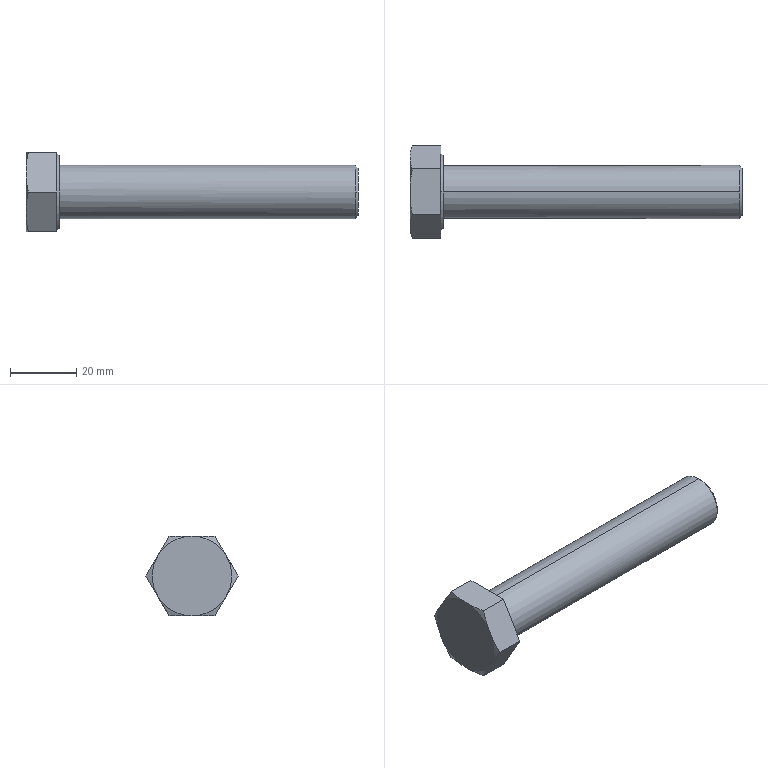Part | STEP file | hex head bolts-full thread grade c gb_GB_FASTENER_BOLT_HHBFTC M16X90-S | 1 solid | 22 faces | box 100 x 27.713 x 24 mm | volume 22987 mm3 | cone 10 | plane 10 | cylinder 2 | commonest cylinder face diameters 16 x2
STEP:
#1=CARTESIAN_POINT('',(99.2,8.,0.));
#2=VERTEX_POINT('',#1);
#3=CARTESIAN_POINT('',(99.2,0.,-8.));
#4=VERTEX_POINT('',#3);
#5=CARTESIAN_POINT('',(99.2,0.,0.));
#6=DIRECTION('',(-1.,0.,0.));
#7=DIRECTION('',(0.,0.,1.));
#8=AXIS2_PLACEMENT_3D('',#5,#6,#7);
#9=CIRCLE('',#8,8.);
#10=EDGE_CURVE('',#2,#4,#9,.T.);
#11=ORIENTED_EDGE('',*,*,#10,.T.);
#12=CARTESIAN_POINT('',(10.,0.,-8.));
#13=VERTEX_POINT('',#12);
#14=CARTESIAN_POINT('',(100.,0.,-8.));
#15=DIRECTION('',(-1.,0.,0.));
#16=VECTOR('',#15,1000.);
#17=LINE('',#14,#16);
#18=EDGE_CURVE('',#4,#13,#17,.T.);
#19=ORIENTED_EDGE('',*,*,#18,.T.);
#20=CARTESIAN_POINT('',(10.,0.,8.));
#21=VERTEX_POINT('',#20);
#22=CARTESIAN_POINT('',(10.,0.,0.));
#23=DIRECTION('',(1.,0.,0.));
#24=DIRECTION('',(0.,0.,1.));
#25=AXIS2_PLACEMENT_3D('',#22,#23,#24);
#26=CIRCLE('',#25,8.);
#27=EDGE_CURVE('',#13,#21,#26,.T.);
#28=ORIENTED_EDGE('',*,*,#27,.T.);
#29=CARTESIAN_POINT('',(99.2,0.,8.));
#30=VERTEX_POINT('',#29);
#31=CARTESIAN_POINT('',(100.,0.,8.));
#32=DIRECTION('',(-1.,0.,0.));
#33=VECTOR('',#32,1000.);
#34=LINE('',#31,#33);
#35=EDGE_CURVE('',#30,#21,#34,.T.);
#36=ORIENTED_EDGE('',*,*,#35,.F.);
#37=CARTESIAN_POINT('',(99.2,0.,0.));
#38=DIRECTION('',(-1.,0.,0.));
#39=DIRECTION('',(0.,0.,1.));
#40=AXIS2_PLACEMENT_3D('',#37,#38,#39);
#41=CIRCLE('',#40,8.);
#42=EDGE_CURVE('',#30,#2,#41,.T.);
#43=ORIENTED_EDGE('',*,*,#42,.T.);
#44=EDGE_LOOP('',(#11,#19,#28,#36,#43));
#45=FACE_OUTER_BOUND('',#44,.T.);
#46=CARTESIAN_POINT('',(100.,0.,0.));
#47=DIRECTION('',(-1.,0.,0.));
#48=DIRECTION('',(0.,0.,1.));
#49=AXIS2_PLACEMENT_3D('',#46,#47,#48);
#50=CYLINDRICAL_SURFACE('',#49,8.);
#51=ADVANCED_FACE('',(#45),#50,.T.);
#52=CARTESIAN_POINT('',(100.,-7.2,0.));
#53=VERTEX_POINT('',#52);
#54=CARTESIAN_POINT('',(100.,7.2,0.));
#55=VERTEX_POINT('',#54);
#56=CARTESIAN_POINT('',(100.,0.,0.));
#57=DIRECTION('',(-1.,0.,0.));
#58=DIRECTION('',(0.,-1.,0.));
#59=AXIS2_PLACEMENT_3D('',#56,#57,#58);
#60=CIRCLE('',#59,7.2);
#61=EDGE_CURVE('',#53,#55,#60,.T.);
#62=ORIENTED_EDGE('',*,*,#61,.T.);
#63=CARTESIAN_POINT('',(99.2,8.,0.));
#64=DIRECTION('',(-0.7071,0.7071,0.));
#65=VECTOR('',#64,1000.);
#66=LINE('',#63,#65);
#67=EDGE_CURVE('',#55,#2,#66,.T.);
#68=ORIENTED_EDGE('',*,*,#67,.T.);
#69=ORIENTED_EDGE('',*,*,#42,.F.);
#70=CARTESIAN_POINT('',(99.2,-8.,0.));
#71=VERTEX_POINT('',#70);
#72=CARTESIAN_POINT('',(99.2,0.,0.));
#73=DIRECTION('',(-1.,0.,0.));
#74=DIRECTION('',(0.,0.,1.));
#75=AXIS2_PLACEMENT_3D('',#72,#73,#74);
#76=CIRCLE('',#75,8.);
#77=EDGE_CURVE('',#71,#30,#76,.T.);
#78=ORIENTED_EDGE('',*,*,#77,.F.);
#79=CARTESIAN_POINT('',(99.2,-8.,0.));
#80=DIRECTION('',(-0.7071,-0.7071,0.));
#81=VECTOR('',#80,1000.);
#82=LINE('',#79,#81);
#83=EDGE_CURVE('',#53,#71,#82,.T.);
#84=ORIENTED_EDGE('',*,*,#83,.F.);
#85=EDGE_LOOP('',(#62,#68,#69,#78,#84));
#86=FACE_OUTER_BOUND('',#85,.T.);
#87=CARTESIAN_POINT('',(99.2,0.,0.));
#88=DIRECTION('',(-1.,0.,0.));
#89=DIRECTION('',(0.,-1.,0.));
#90=AXIS2_PLACEMENT_3D('',#87,#88,#89);
#91=CONICAL_SURFACE('',#90,8.,0.7854);
#92=ADVANCED_FACE('',(#86),#91,.T.);
#93=CARTESIAN_POINT('',(10.,0.,11.));
#94=VERTEX_POINT('',#93);
#95=CARTESIAN_POINT('',(10.,0.,-11.));
#96=VERTEX_POINT('',#95);
#97=CARTESIAN_POINT('',(10.,0.,0.));
#98=DIRECTION('',(-1.,0.,0.));
#99=DIRECTION('',(0.,0.,1.));
#100=AXIS2_PLACEMENT_3D('',#97,#98,#99);
#101=CIRCLE('',#100,11.);
#102=EDGE_CURVE('',#94,#96,#101,.T.);
#103=ORIENTED_EDGE('',*,*,#102,.T.);
#104=CARTESIAN_POINT('',(9.2,0.,-11.8));
#105=VERTEX_POINT('',#104);
#106=CARTESIAN_POINT('',(9.2,0.,-11.8));
#107=DIRECTION('',(-0.7071,0.,-0.7071));
#108=VECTOR('',#107,1000.);
#109=LINE('',#106,#108);
#110=EDGE_CURVE('',#96,#105,#109,.T.);
#111=ORIENTED_EDGE('',*,*,#110,.T.);
#112=CARTESIAN_POINT('',(9.2,0.,11.8));
#113=VERTEX_POINT('',#112);
#114=CARTESIAN_POINT('',(9.2,0.,0.));
#115=DIRECTION('',(1.,0.,0.));
#116=DIRECTION('',(0.,0.,1.));
#117=AXIS2_PLACEMENT_3D('',#114,#115,#116);
#118=CIRCLE('',#117,11.8);
#119=EDGE_CURVE('',#105,#113,#118,.T.);
#120=ORIENTED_EDGE('',*,*,#119,.T.);
#121=CARTESIAN_POINT('',(9.2,0.,11.8));
#122=DIRECTION('',(-0.7071,0.,0.7071));
#123=VECTOR('',#122,1000.);
#124=LINE('',#121,#123);
#125=EDGE_CURVE('',#94,#113,#124,.T.);
#126=ORIENTED_EDGE('',*,*,#125,.F.);
#127=EDGE_LOOP('',(#103,#111,#120,#126));
#128=FACE_OUTER_BOUND('',#127,.T.);
#129=CARTESIAN_POINT('',(9.2,0.,0.));
#130=DIRECTION('',(-1.,0.,0.));
#131=DIRECTION('',(0.,0.,1.));
#132=AXIS2_PLACEMENT_3D('',#129,#130,#131);
#133=CONICAL_SURFACE('',#132,11.8,0.7854);
#134=ADVANCED_FACE('',(#128),#133,.T.);
#135=ORIENTED_EDGE('',*,*,#18,.F.);
#136=CARTESIAN_POINT('',(99.2,0.,0.));
#137=DIRECTION('',(-1.,0.,0.));
#138=DIRECTION('',(0.,0.,1.));
#139=AXIS2_PLACEMENT_3D('',#136,#137,#138);
#140=CIRCLE('',#139,8.);
#141=EDGE_CURVE('',#4,#71,#140,.T.);
#142=ORIENTED_EDGE('',*,*,#141,.T.);
#143=ORIENTED_EDGE('',*,*,#77,.T.);
#144=ORIENTED_EDGE('',*,*,#35,.T.);
#145=CARTESIAN_POINT('',(10.,0.,0.));
#146=DIRECTION('',(1.,0.,0.));
#147=DIRECTION('',(0.,0.,1.));
#148=AXIS2_PLACEMENT_3D('',#145,#146,#147);
#149=CIRCLE('',#148,8.);
#150=EDGE_CURVE('',#21,#13,#149,.T.);
#151=ORIENTED_EDGE('',*,*,#150,.T.);
#152=EDGE_LOOP('',(#135,#142,#143,#144,#151));
#153=FACE_OUTER_BOUND('',#152,.T.);
#154=CARTESIAN_POINT('',(100.,0.,0.));
#155=DIRECTION('',(-1.,0.,0.));
#156=DIRECTION('',(0.,0.,1.));
#157=AXIS2_PLACEMENT_3D('',#154,#155,#156);
#158=CYLINDRICAL_SURFACE('',#157,8.);
#159=ADVANCED_FACE('',(#153),#158,.T.);
#160=ORIENTED_EDGE('',*,*,#150,.F.);
#161=ORIENTED_EDGE('',*,*,#27,.F.);
#162=EDGE_LOOP('',(#160,#161));
#163=FACE_BOUND('',#162,.T.);
#164=ORIENTED_EDGE('',*,*,#102,.F.);
#165=CARTESIAN_POINT('',(10.,0.,0.));
#166=DIRECTION('',(-1.,0.,0.));
#167=DIRECTION('',(0.,0.,1.));
#168=AXIS2_PLACEMENT_3D('',#165,#166,#167);
#169=CIRCLE('',#168,11.);
#170=EDGE_CURVE('',#96,#94,#169,.T.);
#171=ORIENTED_EDGE('',*,*,#170,.F.);
#172=EDGE_LOOP('',(#164,#171));
#173=FACE_OUTER_BOUND('',#172,.T.);
#174=CARTESIAN_POINT('',(10.,0.,24.));
#175=DIRECTION('',(-1.,0.,0.));
#176=DIRECTION('',(0.,0.,1.));
#177=AXIS2_PLACEMENT_3D('',#174,#175,#176);
#178=PLANE('',#177);
#179=ADVANCED_FACE('',(#163,#173),#178,.F.);
#180=ORIENTED_EDGE('',*,*,#67,.F.);
#181=CARTESIAN_POINT('',(100.,0.,0.));
#182=DIRECTION('',(-1.,0.,0.));
#183=DIRECTION('',(0.,-1.,0.));
#184=AXIS2_PLACEMENT_3D('',#181,#182,#183);
#185=CIRCLE('',#184,7.2);
#186=EDGE_CURVE('',#55,#53,#185,.T.);
#187=ORIENTED_EDGE('',*,*,#186,.T.);
#188=ORIENTED_EDGE('',*,*,#83,.T.);
#189=ORIENTED_EDGE('',*,*,#141,.F.);
#190=ORIENTED_EDGE('',*,*,#10,.F.);
#191=EDGE_LOOP('',(#180,#187,#188,#189,#190));
#192=FACE_OUTER_BOUND('',#191,.T.);
#193=CARTESIAN_POINT('',(99.2,0.,0.));
#194=DIRECTION('',(-1.,0.,0.));
#195=DIRECTION('',(0.,-1.,0.));
#196=AXIS2_PLACEMENT_3D('',#193,#194,#195);
#197=CONICAL_SURFACE('',#196,8.,0.7854);
#198=ADVANCED_FACE('',(#192),#197,.T.);
#199=ORIENTED_EDGE('',*,*,#110,.F.);
#200=ORIENTED_EDGE('',*,*,#170,.T.);
#201=ORIENTED_EDGE('',*,*,#125,.T.);
#202=CARTESIAN_POINT('',(9.2,0.,0.));
#203=DIRECTION('',(1.,0.,0.));
#204=DIRECTION('',(0.,0.,1.));
#205=AXIS2_PLACEMENT_3D('',#202,#203,#204);
#206=CIRCLE('',#205,11.8);
#207=EDGE_CURVE('',#113,#105,#206,.T.);
#208=ORIENTED_EDGE('',*,*,#207,.T.);
#209=EDGE_LOOP('',(#199,#200,#201,#208));
#210=FACE_OUTER_BOUND('',#209,.T.);
#211=CARTESIAN_POINT('',(9.2,0.,0.));
#212=DIRECTION('',(-1.,0.,0.));
#213=DIRECTION('',(0.,0.,1.));
#214=AXIS2_PLACEMENT_3D('',#211,#212,#213);
#215=CONICAL_SURFACE('',#214,11.8,0.7854);
#216=ADVANCED_FACE('',(#210),#215,.T.);
#217=ORIENTED_EDGE('',*,*,#61,.F.);
#218=ORIENTED_EDGE('',*,*,#186,.F.);
#219=EDGE_LOOP('',(#217,#218));
#220=FACE_OUTER_BOUND('',#219,.T.);
#221=CARTESIAN_POINT('',(100.,0.,0.));
#222=DIRECTION('',(1.,0.,0.));
#223=DIRECTION('',(0.,0.,-1.));
#224=AXIS2_PLACEMENT_3D('',#221,#222,#223);
#225=PLANE('',#224);
#226=ADVANCED_FACE('',(#220),#225,.T.);
#227=CARTESIAN_POINT('',(9.2,13.856,0.));
#228=VERTEX_POINT('',#227);
#229=CARTESIAN_POINT('',(9.2,6.928,12.));
#230=VERTEX_POINT('',#229);
#231=CARTESIAN_POINT('',(9.2,13.856,0.));
#232=DIRECTION('',(0.,-0.5,0.866));
#233=VECTOR('',#232,1000.);
#234=LINE('',#231,#233);
#235=EDGE_CURVE('',#228,#230,#234,.T.);
#236=ORIENTED_EDGE('',*,*,#235,.T.);
#237=CARTESIAN_POINT('',(9.2,-6.928,12.));
#238=VERTEX_POINT('',#237);
#239=CARTESIAN_POINT('',(9.2,11.8,12.));
#240=DIRECTION('',(0.,-1.,0.));
#241=VECTOR('',#240,1000.);
#242=LINE('',#239,#241);
#243=EDGE_CURVE('',#230,#238,#242,.T.);
#244=ORIENTED_EDGE('',*,*,#243,.T.);
#245=CARTESIAN_POINT('',(9.2,-13.856,0.));
#246=VERTEX_POINT('',#245);
#247=CARTESIAN_POINT('',(9.2,-6.928,12.));
#248=DIRECTION('',(0.,-0.5,-0.866));
#249=VECTOR('',#248,1000.);
#250=LINE('',#247,#249);
#251=EDGE_CURVE('',#238,#246,#250,.T.);
#252=ORIENTED_EDGE('',*,*,#251,.T.);
#253=CARTESIAN_POINT('',(9.2,-6.928,-12.));
#254=VERTEX_POINT('',#253);
#255=CARTESIAN_POINT('',(9.2,-13.856,0.));
#256=DIRECTION('',(0.,0.5,-0.866));
#257=VECTOR('',#256,1000.);
#258=LINE('',#255,#257);
#259=EDGE_CURVE('',#246,#254,#258,.T.);
#260=ORIENTED_EDGE('',*,*,#259,.T.);
#261=CARTESIAN_POINT('',(9.2,6.928,-12.));
#262=VERTEX_POINT('',#261);
#263=CARTESIAN_POINT('',(9.2,11.8,-12.));
#264=DIRECTION('',(0.,1.,0.));
#265=VECTOR('',#264,1000.);
#266=LINE('',#263,#265);
#267=EDGE_CURVE('',#254,#262,#266,.T.);
#268=ORIENTED_EDGE('',*,*,#267,.T.);
#269=CARTESIAN_POINT('',(9.2,6.928,-12.));
#270=DIRECTION('',(0.,0.5,0.866));
#271=VECTOR('',#270,1000.);
#272=LINE('',#269,#271);
#273=EDGE_CURVE('',#262,#228,#272,.T.);
#274=ORIENTED_EDGE('',*,*,#273,.T.);
#275=EDGE_LOOP('',(#236,#244,#252,#260,#268,#274));
#276=FACE_OUTER_BOUND('',#275,.T.);
#277=ORIENTED_EDGE('',*,*,#207,.F.);
#278=ORIENTED_EDGE('',*,*,#119,.F.);
#279=EDGE_LOOP('',(#277,#278));
#280=FACE_BOUND('',#279,.T.);
#281=CARTESIAN_POINT('',(9.2,11.8,0.));
#282=DIRECTION('',(1.,0.,0.));
#283=DIRECTION('',(0.,0.,-1.));
#284=AXIS2_PLACEMENT_3D('',#281,#282,#283);
#285=PLANE('',#284);
#286=ADVANCED_FACE('',(#276,#280),#285,.T.);
#287=CARTESIAN_POINT('',(0.6757,-6.928,12.));
#288=VERTEX_POINT('',#287);
#289=CARTESIAN_POINT('',(10.,-6.928,12.));
#290=DIRECTION('',(-1.,0.,0.));
#291=VECTOR('',#290,1000.);
#292=LINE('',#289,#291);
#293=EDGE_CURVE('',#238,#288,#292,.T.);
#294=ORIENTED_EDGE('',*,*,#293,.F.);
#295=ORIENTED_EDGE('',*,*,#243,.F.);
#296=CARTESIAN_POINT('',(0.6757,6.928,12.));
#297=VERTEX_POINT('',#296);
#298=CARTESIAN_POINT('',(10.,6.928,12.));
#299=DIRECTION('',(1.,0.,0.));
#300=VECTOR('',#299,1000.);
#301=LINE('',#298,#300);
#302=EDGE_CURVE('',#297,#230,#301,.T.);
#303=ORIENTED_EDGE('',*,*,#302,.F.);
#304=CARTESIAN_POINT('',(0.,0.,12.));
#305=VERTEX_POINT('',#304);
#306=CARTESIAN_POINT('',(0.,0.,12.));
#307=CARTESIAN_POINT('',(0.,1.166,12.));
#308=CARTESIAN_POINT('',(0.0629,2.325,12.));
#309=CARTESIAN_POINT('',(0.2969,4.634,12.));
#310=CARTESIAN_POINT('',(0.4672,5.783,12.));
#311=CARTESIAN_POINT('',(0.6757,6.928,12.));
#312=B_SPLINE_CURVE_WITH_KNOTS('',3,(#306,#307,#308,#309,#310,#311),.UNSPECIFIED.,.F.,.F.,(4,2,4),(0.,0.003481,0.006961),.UNSPECIFIED.);
#313=EDGE_CURVE('',#305,#297,#312,.T.);
#314=ORIENTED_EDGE('',*,*,#313,.F.);
#315=CARTESIAN_POINT('',(0.6757,-6.928,12.));
#316=CARTESIAN_POINT('',(0.4672,-5.783,12.));
#317=CARTESIAN_POINT('',(0.2969,-4.634,12.));
#318=CARTESIAN_POINT('',(0.0629,-2.325,12.));
#319=CARTESIAN_POINT('',(0.,-1.166,12.));
#320=CARTESIAN_POINT('',(0.,0.,12.));
#321=B_SPLINE_CURVE_WITH_KNOTS('',3,(#315,#316,#317,#318,#319,#320),.UNSPECIFIED.,.F.,.F.,(4,2,4),(0.,0.003481,0.006961),.UNSPECIFIED.);
#322=EDGE_CURVE('',#288,#305,#321,.T.);
#323=ORIENTED_EDGE('',*,*,#322,.F.);
#324=EDGE_LOOP('',(#294,#295,#303,#314,#323));
#325=FACE_OUTER_BOUND('',#324,.T.);
#326=CARTESIAN_POINT('',(10.,6.928,12.));
#327=DIRECTION('',(0.,0.,-1.));
#328=DIRECTION('',(-1.,0.,0.));
#329=AXIS2_PLACEMENT_3D('',#326,#327,#328);
#330=PLANE('',#329);
#331=ADVANCED_FACE('',(#325),#330,.F.);
#332=ORIENTED_EDGE('',*,*,#302,.T.);
#333=ORIENTED_EDGE('',*,*,#235,.F.);
#334=CARTESIAN_POINT('',(0.6757,13.856,0.));
#335=VERTEX_POINT('',#334);
#336=CARTESIAN_POINT('',(10.,13.856,0.));
#337=DIRECTION('',(1.,0.,0.));
#338=VECTOR('',#337,1000.);
#339=LINE('',#336,#338);
#340=EDGE_CURVE('',#335,#228,#339,.T.);
#341=ORIENTED_EDGE('',*,*,#340,.F.);
#342=CARTESIAN_POINT('',(0.,10.392,6.));
#343=VERTEX_POINT('',#342);
#344=CARTESIAN_POINT('',(0.,10.392,6.));
#345=CARTESIAN_POINT('',(0.,10.975,4.99));
#346=CARTESIAN_POINT('',(0.0629,11.555,3.986));
#347=CARTESIAN_POINT('',(0.2969,12.709,1.987));
#348=CARTESIAN_POINT('',(0.4672,13.284,0.9919));
#349=CARTESIAN_POINT('',(0.6757,13.856,0.));
#350=B_SPLINE_CURVE_WITH_KNOTS('',3,(#344,#345,#346,#347,#348,#349),.UNSPECIFIED.,.F.,.F.,(4,2,4),(0.,0.003481,0.006961),.UNSPECIFIED.);
#351=EDGE_CURVE('',#343,#335,#350,.T.);
#352=ORIENTED_EDGE('',*,*,#351,.F.);
#353=CARTESIAN_POINT('',(0.6757,6.928,12.));
#354=CARTESIAN_POINT('',(0.4672,7.501,11.008));
#355=CARTESIAN_POINT('',(0.2969,8.075,10.013));
#356=CARTESIAN_POINT('',(0.0629,9.23,8.014));
#357=CARTESIAN_POINT('',(0.,9.809,7.01));
#358=CARTESIAN_POINT('',(0.,10.392,6.));
#359=B_SPLINE_CURVE_WITH_KNOTS('',3,(#353,#354,#355,#356,#357,#358),.UNSPECIFIED.,.F.,.F.,(4,2,4),(0.,0.003481,0.006961),.UNSPECIFIED.);
#360=EDGE_CURVE('',#297,#343,#359,.T.);
#361=ORIENTED_EDGE('',*,*,#360,.F.);
#362=EDGE_LOOP('',(#332,#333,#341,#352,#361));
#363=FACE_OUTER_BOUND('',#362,.T.);
#364=CARTESIAN_POINT('',(10.,13.856,0.));
#365=DIRECTION('',(0.,-0.866,-0.5));
#366=DIRECTION('',(0.,0.5,-0.866));
#367=AXIS2_PLACEMENT_3D('',#364,#365,#366);
#368=PLANE('',#367);
#369=ADVANCED_FACE('',(#363),#368,.F.);
#370=ORIENTED_EDGE('',*,*,#340,.T.);
#371=ORIENTED_EDGE('',*,*,#273,.F.);
#372=CARTESIAN_POINT('',(0.6757,6.928,-12.));
#373=VERTEX_POINT('',#372);
#374=CARTESIAN_POINT('',(10.,6.928,-12.));
#375=DIRECTION('',(1.,0.,0.));
#376=VECTOR('',#375,1000.);
#377=LINE('',#374,#376);
#378=EDGE_CURVE('',#373,#262,#377,.T.);
#379=ORIENTED_EDGE('',*,*,#378,.F.);
#380=CARTESIAN_POINT('',(0.,10.392,-6.));
#381=VERTEX_POINT('',#380);
#382=CARTESIAN_POINT('',(0.,10.392,-6.));
#383=CARTESIAN_POINT('',(0.,9.809,-7.01));
#384=CARTESIAN_POINT('',(0.0629,9.23,-8.014));
#385=CARTESIAN_POINT('',(0.2969,8.075,-10.013));
#386=CARTESIAN_POINT('',(0.4672,7.501,-11.008));
#387=CARTESIAN_POINT('',(0.6757,6.928,-12.));
#388=B_SPLINE_CURVE_WITH_KNOTS('',3,(#382,#383,#384,#385,#386,#387),.UNSPECIFIED.,.F.,.F.,(4,2,4),(0.,0.003481,0.006961),.UNSPECIFIED.);
#389=EDGE_CURVE('',#381,#373,#388,.T.);
#390=ORIENTED_EDGE('',*,*,#389,.F.);
#391=CARTESIAN_POINT('',(0.6757,13.856,0.));
#392=CARTESIAN_POINT('',(0.4672,13.284,-0.9919));
#393=CARTESIAN_POINT('',(0.2969,12.709,-1.987));
#394=CARTESIAN_POINT('',(0.0629,11.555,-3.986));
#395=CARTESIAN_POINT('',(0.,10.975,-4.99));
#396=CARTESIAN_POINT('',(0.,10.392,-6.));
#397=B_SPLINE_CURVE_WITH_KNOTS('',3,(#391,#392,#393,#394,#395,#396),.UNSPECIFIED.,.F.,.F.,(4,2,4),(0.,0.003481,0.006961),.UNSPECIFIED.);
#398=EDGE_CURVE('',#335,#381,#397,.T.);
#399=ORIENTED_EDGE('',*,*,#398,.F.);
#400=EDGE_LOOP('',(#370,#371,#379,#390,#399));
#401=FACE_OUTER_BOUND('',#400,.T.);
#402=CARTESIAN_POINT('',(10.,6.928,-12.));
#403=DIRECTION('',(0.,-0.866,0.5));
#404=DIRECTION('',(0.,-0.5,-0.866));
#405=AXIS2_PLACEMENT_3D('',#402,#403,#404);
#406=PLANE('',#405);
#407=ADVANCED_FACE('',(#401),#406,.F.);
#408=ORIENTED_EDGE('',*,*,#378,.T.);
#409=ORIENTED_EDGE('',*,*,#267,.F.);
#410=CARTESIAN_POINT('',(0.6757,-6.928,-12.));
#411=VERTEX_POINT('',#410);
#412=CARTESIAN_POINT('',(10.,-6.928,-12.));
#413=DIRECTION('',(1.,0.,0.));
#414=VECTOR('',#413,1000.);
#415=LINE('',#412,#414);
#416=EDGE_CURVE('',#411,#254,#415,.T.);
#417=ORIENTED_EDGE('',*,*,#416,.F.);
#418=CARTESIAN_POINT('',(0.,0.,-12.));
#419=VERTEX_POINT('',#418);
#420=CARTESIAN_POINT('',(0.,0.,-12.));
#421=CARTESIAN_POINT('',(0.,-1.166,-12.));
#422=CARTESIAN_POINT('',(0.0629,-2.325,-12.));
#423=CARTESIAN_POINT('',(0.2969,-4.634,-12.));
#424=CARTESIAN_POINT('',(0.4672,-5.783,-12.));
#425=CARTESIAN_POINT('',(0.6757,-6.928,-12.));
#426=B_SPLINE_CURVE_WITH_KNOTS('',3,(#420,#421,#422,#423,#424,#425),.UNSPECIFIED.,.F.,.F.,(4,2,4),(0.,0.003481,0.006961),.UNSPECIFIED.);
#427=EDGE_CURVE('',#419,#411,#426,.T.);
#428=ORIENTED_EDGE('',*,*,#427,.F.);
#429=CARTESIAN_POINT('',(0.6757,6.928,-12.));
#430=CARTESIAN_POINT('',(0.4672,5.783,-12.));
#431=CARTESIAN_POINT('',(0.2969,4.634,-12.));
#432=CARTESIAN_POINT('',(0.0629,2.325,-12.));
#433=CARTESIAN_POINT('',(0.,1.166,-12.));
#434=CARTESIAN_POINT('',(0.,0.,-12.));
#435=B_SPLINE_CURVE_WITH_KNOTS('',3,(#429,#430,#431,#432,#433,#434),.UNSPECIFIED.,.F.,.F.,(4,2,4),(0.,0.003481,0.006961),.UNSPECIFIED.);
#436=EDGE_CURVE('',#373,#419,#435,.T.);
#437=ORIENTED_EDGE('',*,*,#436,.F.);
#438=EDGE_LOOP('',(#408,#409,#417,#428,#437));
#439=FACE_OUTER_BOUND('',#438,.T.);
#440=CARTESIAN_POINT('',(10.,-6.928,-12.));
#441=DIRECTION('',(0.,0.,1.));
#442=DIRECTION('',(0.,-1.,0.));
#443=AXIS2_PLACEMENT_3D('',#440,#441,#442);
#444=PLANE('',#443);
#445=ADVANCED_FACE('',(#439),#444,.F.);
#446=ORIENTED_EDGE('',*,*,#416,.T.);
#447=ORIENTED_EDGE('',*,*,#259,.F.);
#448=CARTESIAN_POINT('',(0.6757,-13.856,0.));
#449=VERTEX_POINT('',#448);
#450=CARTESIAN_POINT('',(10.,-13.856,0.));
#451=DIRECTION('',(1.,0.,0.));
#452=VECTOR('',#451,1000.);
#453=LINE('',#450,#452);
#454=EDGE_CURVE('',#449,#246,#453,.T.);
#455=ORIENTED_EDGE('',*,*,#454,.F.);
#456=CARTESIAN_POINT('',(0.,-10.392,-6.));
#457=VERTEX_POINT('',#456);
#458=CARTESIAN_POINT('',(0.,-10.392,-6.));
#459=CARTESIAN_POINT('',(0.,-10.975,-4.99));
#460=CARTESIAN_POINT('',(0.0629,-11.555,-3.986));
#461=CARTESIAN_POINT('',(0.2969,-12.709,-1.987));
#462=CARTESIAN_POINT('',(0.4672,-13.284,-0.9919));
#463=CARTESIAN_POINT('',(0.6757,-13.856,0.));
#464=B_SPLINE_CURVE_WITH_KNOTS('',3,(#458,#459,#460,#461,#462,#463),.UNSPECIFIED.,.F.,.F.,(4,2,4),(0.,0.003481,0.006961),.UNSPECIFIED.);
#465=EDGE_CURVE('',#457,#449,#464,.T.);
#466=ORIENTED_EDGE('',*,*,#465,.F.);
#467=CARTESIAN_POINT('',(0.6757,-6.928,-12.));
#468=CARTESIAN_POINT('',(0.4672,-7.501,-11.008));
#469=CARTESIAN_POINT('',(0.2969,-8.075,-10.013));
#470=CARTESIAN_POINT('',(0.0629,-9.23,-8.014));
#471=CARTESIAN_POINT('',(0.,-9.809,-7.01));
#472=CARTESIAN_POINT('',(0.,-10.392,-6.));
#473=B_SPLINE_CURVE_WITH_KNOTS('',3,(#467,#468,#469,#470,#471,#472),.UNSPECIFIED.,.F.,.F.,(4,2,4),(0.,0.003481,0.006961),.UNSPECIFIED.);
#474=EDGE_CURVE('',#411,#457,#473,.T.);
#475=ORIENTED_EDGE('',*,*,#474,.F.);
#476=EDGE_LOOP('',(#446,#447,#455,#466,#475));
#477=FACE_OUTER_BOUND('',#476,.T.);
#478=CARTESIAN_POINT('',(10.,-13.856,0.));
#479=DIRECTION('',(0.,0.866,0.5));
#480=DIRECTION('',(0.,-0.5,0.866));
#481=AXIS2_PLACEMENT_3D('',#478,#479,#480);
#482=PLANE('',#481);
#483=ADVANCED_FACE('',(#477),#482,.F.);
#484=ORIENTED_EDGE('',*,*,#454,.T.);
#485=ORIENTED_EDGE('',*,*,#251,.F.);
#486=ORIENTED_EDGE('',*,*,#293,.T.);
#487=CARTESIAN_POINT('',(0.,-10.392,6.));
#488=VERTEX_POINT('',#487);
#489=CARTESIAN_POINT('',(0.,-10.392,6.));
#490=CARTESIAN_POINT('',(0.,-9.809,7.01));
#491=CARTESIAN_POINT('',(0.0629,-9.23,8.014));
#492=CARTESIAN_POINT('',(0.2969,-8.075,10.013));
#493=CARTESIAN_POINT('',(0.4672,-7.501,11.008));
#494=CARTESIAN_POINT('',(0.6757,-6.928,12.));
#495=B_SPLINE_CURVE_WITH_KNOTS('',3,(#489,#490,#491,#492,#493,#494),.UNSPECIFIED.,.F.,.F.,(4,2,4),(0.,0.003481,0.006961),.UNSPECIFIED.);
#496=EDGE_CURVE('',#488,#288,#495,.T.);
#497=ORIENTED_EDGE('',*,*,#496,.F.);
#498=CARTESIAN_POINT('',(0.6757,-13.856,0.));
#499=CARTESIAN_POINT('',(0.4672,-13.284,0.9919));
#500=CARTESIAN_POINT('',(0.2969,-12.709,1.987));
#501=CARTESIAN_POINT('',(0.0629,-11.555,3.986));
#502=CARTESIAN_POINT('',(0.,-10.975,4.99));
#503=CARTESIAN_POINT('',(0.,-10.392,6.));
#504=B_SPLINE_CURVE_WITH_KNOTS('',3,(#498,#499,#500,#501,#502,#503),.UNSPECIFIED.,.F.,.F.,(4,2,4),(0.,0.003481,0.006961),.UNSPECIFIED.);
#505=EDGE_CURVE('',#449,#488,#504,.T.);
#506=ORIENTED_EDGE('',*,*,#505,.F.);
#507=EDGE_LOOP('',(#484,#485,#486,#497,#506));
#508=FACE_OUTER_BOUND('',#507,.T.);
#509=CARTESIAN_POINT('',(10.,-6.928,12.));
#510=DIRECTION('',(0.,0.866,-0.5));
#511=DIRECTION('',(0.,0.5,0.866));
#512=AXIS2_PLACEMENT_3D('',#509,#510,#511);
#513=PLANE('',#512);
#514=ADVANCED_FACE('',(#508),#513,.F.);
#515=ORIENTED_EDGE('',*,*,#322,.T.);
#516=CARTESIAN_POINT('',(0.,0.,0.));
#517=DIRECTION('',(1.,0.,0.));
#518=DIRECTION('',(0.,0.,-1.));
#519=AXIS2_PLACEMENT_3D('',#516,#517,#518);
#520=CIRCLE('',#519,12.);
#521=EDGE_CURVE('',#305,#488,#520,.T.);
#522=ORIENTED_EDGE('',*,*,#521,.T.);
#523=ORIENTED_EDGE('',*,*,#496,.T.);
#524=EDGE_LOOP('',(#515,#522,#523));
#525=FACE_OUTER_BOUND('',#524,.T.);
#526=CARTESIAN_POINT('',(0.6797,0.,0.));
#527=DIRECTION('',(1.,0.,0.));
#528=DIRECTION('',(0.,0.,-1.));
#529=AXIS2_PLACEMENT_3D('',#526,#527,#528);
#530=CONICAL_SURFACE('',#529,13.868,1.222);
#531=ADVANCED_FACE('',(#525),#530,.T.);
#532=CARTESIAN_POINT('',(0.,0.,0.));
#533=DIRECTION('',(1.,0.,0.));
#534=DIRECTION('',(0.,0.,-1.));
#535=AXIS2_PLACEMENT_3D('',#532,#533,#534);
#536=CIRCLE('',#535,12.);
#537=EDGE_CURVE('',#343,#305,#536,.T.);
#538=ORIENTED_EDGE('',*,*,#537,.T.);
#539=ORIENTED_EDGE('',*,*,#313,.T.);
#540=ORIENTED_EDGE('',*,*,#360,.T.);
#541=EDGE_LOOP('',(#538,#539,#540));
#542=FACE_OUTER_BOUND('',#541,.T.);
#543=CARTESIAN_POINT('',(0.6797,0.,0.));
#544=DIRECTION('',(1.,0.,0.));
#545=DIRECTION('',(0.,0.,-1.));
#546=AXIS2_PLACEMENT_3D('',#543,#544,#545);
#547=CONICAL_SURFACE('',#546,13.868,1.222);
#548=ADVANCED_FACE('',(#542),#547,.T.);
#549=CARTESIAN_POINT('',(0.,0.,0.));
#550=DIRECTION('',(1.,0.,0.));
#551=DIRECTION('',(0.,0.,-1.));
#552=AXIS2_PLACEMENT_3D('',#549,#550,#551);
#553=CIRCLE('',#552,12.);
#554=EDGE_CURVE('',#381,#343,#553,.T.);
#555=ORIENTED_EDGE('',*,*,#554,.T.);
#556=ORIENTED_EDGE('',*,*,#351,.T.);
#557=ORIENTED_EDGE('',*,*,#398,.T.);
#558=EDGE_LOOP('',(#555,#556,#557));
#559=FACE_OUTER_BOUND('',#558,.T.);
#560=CARTESIAN_POINT('',(0.6797,0.,0.));
#561=DIRECTION('',(1.,0.,0.));
#562=DIRECTION('',(0.,0.,-1.));
#563=AXIS2_PLACEMENT_3D('',#560,#561,#562);
#564=CONICAL_SURFACE('',#563,13.868,1.222);
#565=ADVANCED_FACE('',(#559),#564,.T.);
#566=CARTESIAN_POINT('',(0.,0.,0.));
#567=DIRECTION('',(1.,0.,0.));
#568=DIRECTION('',(0.,0.,-1.));
#569=AXIS2_PLACEMENT_3D('',#566,#567,#568);
#570=CIRCLE('',#569,12.);
#571=EDGE_CURVE('',#419,#381,#570,.T.);
#572=ORIENTED_EDGE('',*,*,#571,.T.);
#573=ORIENTED_EDGE('',*,*,#389,.T.);
#574=ORIENTED_EDGE('',*,*,#436,.T.);
#575=EDGE_LOOP('',(#572,#573,#574));
#576=FACE_OUTER_BOUND('',#575,.T.);
#577=CARTESIAN_POINT('',(0.6797,0.,0.));
#578=DIRECTION('',(1.,0.,0.));
#579=DIRECTION('',(0.,0.,-1.));
#580=AXIS2_PLACEMENT_3D('',#577,#578,#579);
#581=CONICAL_SURFACE('',#580,13.868,1.222);
#582=ADVANCED_FACE('',(#576),#581,.T.);
#583=ORIENTED_EDGE('',*,*,#474,.T.);
#584=CARTESIAN_POINT('',(0.,0.,0.));
#585=DIRECTION('',(1.,0.,0.));
#586=DIRECTION('',(0.,0.,-1.));
#587=AXIS2_PLACEMENT_3D('',#584,#585,#586);
#588=CIRCLE('',#587,12.);
#589=EDGE_CURVE('',#457,#419,#588,.T.);
#590=ORIENTED_EDGE('',*,*,#589,.T.);
#591=ORIENTED_EDGE('',*,*,#427,.T.);
#592=EDGE_LOOP('',(#583,#590,#591));
#593=FACE_OUTER_BOUND('',#592,.T.);
#594=CARTESIAN_POINT('',(0.6797,0.,0.));
#595=DIRECTION('',(1.,0.,0.));
#596=DIRECTION('',(0.,0.,-1.));
#597=AXIS2_PLACEMENT_3D('',#594,#595,#596);
#598=CONICAL_SURFACE('',#597,13.868,1.222);
#599=ADVANCED_FACE('',(#593),#598,.T.);
#600=ORIENTED_EDGE('',*,*,#505,.T.);
#601=CARTESIAN_POINT('',(0.,0.,0.));
#602=DIRECTION('',(1.,0.,0.));
#603=DIRECTION('',(0.,0.,-1.));
#604=AXIS2_PLACEMENT_3D('',#601,#602,#603);
#605=CIRCLE('',#604,12.);
#606=EDGE_CURVE('',#488,#457,#605,.T.);
#607=ORIENTED_EDGE('',*,*,#606,.T.);
#608=ORIENTED_EDGE('',*,*,#465,.T.);
#609=EDGE_LOOP('',(#600,#607,#608));
#610=FACE_OUTER_BOUND('',#609,.T.);
#611=CARTESIAN_POINT('',(0.6797,0.,0.));
#612=DIRECTION('',(1.,0.,0.));
#613=DIRECTION('',(0.,0.,-1.));
#614=AXIS2_PLACEMENT_3D('',#611,#612,#613);
#615=CONICAL_SURFACE('',#614,13.868,1.222);
#616=ADVANCED_FACE('',(#610),#615,.T.);
#617=ORIENTED_EDGE('',*,*,#589,.F.);
#618=ORIENTED_EDGE('',*,*,#606,.F.);
#619=ORIENTED_EDGE('',*,*,#521,.F.);
#620=ORIENTED_EDGE('',*,*,#537,.F.);
#621=ORIENTED_EDGE('',*,*,#554,.F.);
#622=ORIENTED_EDGE('',*,*,#571,.F.);
#623=EDGE_LOOP('',(#617,#618,#619,#620,#621,#622));
#624=FACE_OUTER_BOUND('',#623,.T.);
#625=CARTESIAN_POINT('',(0.,0.,24.));
#626=DIRECTION('',(-1.,0.,0.));
#627=DIRECTION('',(0.,0.,1.));
#628=AXIS2_PLACEMENT_3D('',#625,#626,#627);
#629=PLANE('',#628);
#630=ADVANCED_FACE('',(#624),#629,.T.);
#631=CLOSED_SHELL('',(#51,#92,#134,#159,#179,#198,#216,#226,#286,#331,#369,#407,#445,#483,#514,#531,#548,#565,#582,#599,#616,#630));
#632=MANIFOLD_SOLID_BREP('',#631);
#633=CARTESIAN_POINT('',(0.,0.,0.));
#634=DIRECTION('',(0.,0.,1.));
#635=DIRECTION('',(1.,0.,0.));
#636=AXIS2_PLACEMENT_3D('',#633,#634,#635);
#637=(LENGTH_UNIT()NAMED_UNIT(*)SI_UNIT(.MILLI.,.METRE.));
#638=UNCERTAINTY_MEASURE_WITH_UNIT(LENGTH_MEASURE(0.00001),#637,'','');
#639=(NAMED_UNIT(*)PLANE_ANGLE_UNIT()SI_UNIT($,.RADIAN.));
#640=(NAMED_UNIT(*)SI_UNIT($,.STERADIAN.)SOLID_ANGLE_UNIT());
#641=(GEOMETRIC_REPRESENTATION_CONTEXT(3)GLOBAL_UNCERTAINTY_ASSIGNED_CONTEXT((#638))GLOBAL_UNIT_ASSIGNED_CONTEXT((#637,#639,#640))REPRESENTATION_CONTEXT('',''));
#642=ADVANCED_BREP_SHAPE_REPRESENTATION('',(#632,#636),#641);